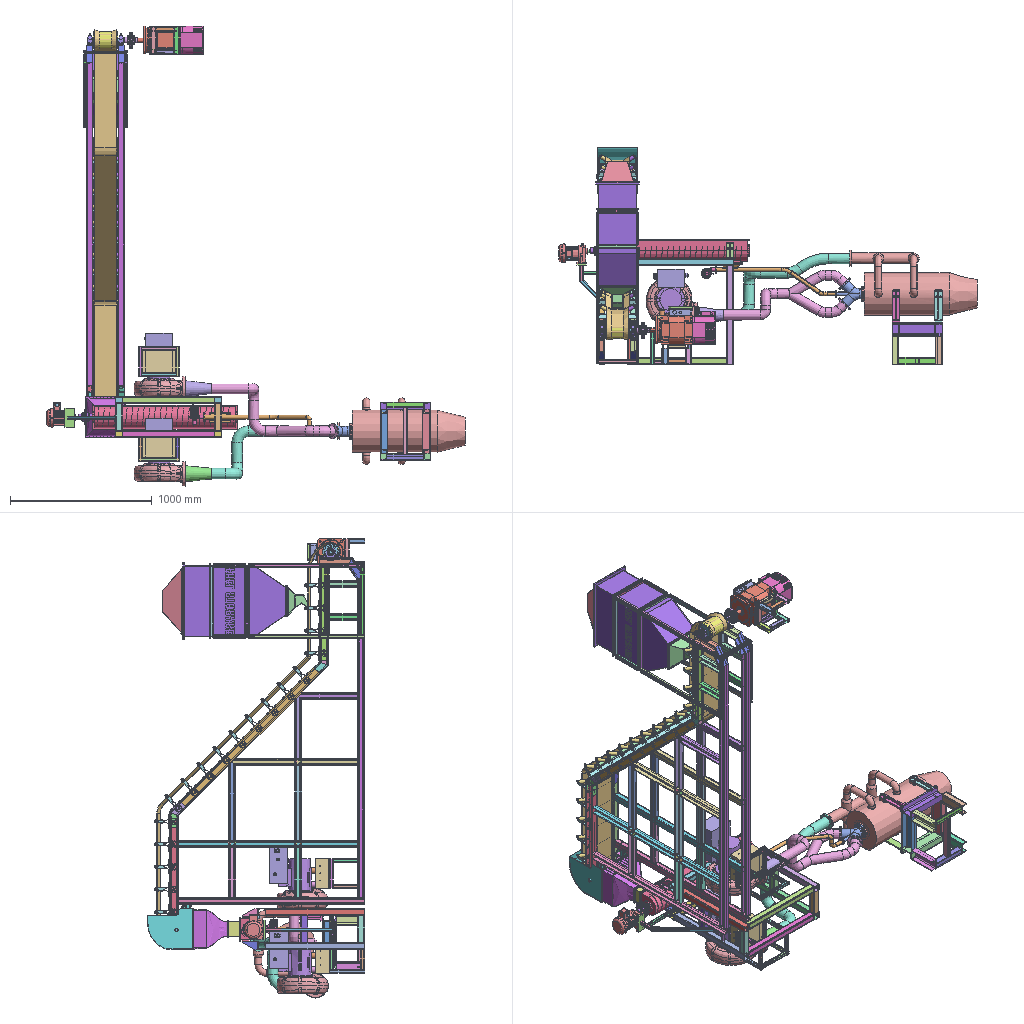Assembly | STEP file | 171 different items | 266 placed | box 2958 x 1534 x 3249 mm
Parts list (item | name | quantity | parent item | size | volume):
1 | 02288023_01 | x4 | in 02288023 | 52 x 34.1 x 52 mm | 26844 mm3
2 | 02288023_02 | x4 | in 02288023 | 140 x 38 x 80.599 mm | 93957 mm3
3 | Coal Storage | x1 | - | 1037 x 540 x 310 mm | 5068760 mm3
4 | Comveyor | x1 | - | - | -
5 | DIN 1026-1 U 30x15 1785506883170 | x1 | in Frame 1784900427749 | 15 x 30 x 530 mm | 112916 mm3
6 | DIN 1026-1 U 30x15 1785506933780 | x1 | in Frame 1784900427749 | 15 x 30 x 300 mm | 62027 mm3
7 | DIN 1026-1 U 30x15 1785506933862 | x1 | in Frame 1784900427749 | 15 x 30 x 530 mm | 112916 mm3
8 | DIN 1026-1 U 30x15 1785506933934 | x1 | in Frame 1784900427749 | 15 x 30 x 300 mm | 62027 mm3
9 | DIN 1026-1 U 30x15 1785506934014 | x1 | in Frame 1784900427749 | 15 x 30 x 530 mm | 112916 mm3
10 | DIN 1026-1 U 30x15 1785506934084 | x1 | in Frame 1784900427749 | 15 x 30 x 300 mm | 62027 mm3
11 | DIN 1026-1 U 30x15 1785506934163 | x1 | in Frame 1784900427749 | 15 x 30 x 530 mm | 112916 mm3
12 | DIN 1026-1 U 30x15 1785506934236 | x1 | in Frame 1784900427749 | 15 x 30 x 300 mm | 62027 mm3
13 | DIN 1026-1 U 30x15 1785507254409 | x1 | in Frame 1784900427749 | 15 x 30 x 815 mm | 180323 mm3
14 | DIN 1026-1 U 30x15 1785507254479 | x1 | in Frame 1784900427749 | 15 x 30 x 815 mm | 180323 mm3
15 | DIN 1026-1 U 30x15 1785507358854 | x1 | in Frame 1784900427749 | 15 x 30 x 815 mm | 180323 mm3
16 | DIN 1026-1 U 30x15 1785507358927 | x1 | in Frame 1784900427749 | 15 x 30 x 815 mm | 180323 mm3
17 | DIN 1026-1 U 30x15 1785507675323 | x1 | in Frame 1784900427749 | 15 x 30 x 470 mm | 103990 mm3
18 | DIN 1026-1 U 30x15 1785507675399 | x1 | in Frame 1784900427749 | 15 x 30 x 470 mm | 103990 mm3
19 | DIN 1026-1 U 30x15 1785507675476 | x1 | in Frame 1784900427749 | 15 x 30 x 270 mm | 59739 mm3
20 | DIN 1026-1 U 30x15 1785507904982 | x1 | in Frame 1784900427749 | 15 x 30 x 470 mm | 103990 mm3
21 | DIN 1026-1 U 30x15 1785507905050 | x1 | in Frame 1784900427749 | 15 x 30 x 470 mm | 103990 mm3
22 | DIN 1026-1 U 30x15 1785508252631 | x1 | in Frame 1784900427749 | 15 x 30 x 220 mm | 48676 mm3
23 | DIN 1026-1 U 30x15 1785508252702 | x1 | in Frame 1784900427749 | 15 x 30 x 220 mm | 48676 mm3
24 | DIN 1026-1 U 30x15 1785508276013 | x1 | in Frame 1784900427749 | 15 x 30 x 220 mm | 48676 mm3
25 | DIN 1026-1 U 30x15 1785508276077 | x1 | in Frame 1784900427749 | 15 x 30 x 220 mm | 48676 mm3
26 | DIN 1026-1 U 50 1785357045320 | x2 | in Frame 1784900427749, Frame 1784900427749_MIR1 | 38 x 50 x 1315 mm | 935965 mm3
27 | DIN 1026-1 U 50 1785357045389 | x2 | in Frame 1784900427749, Frame 1784900427749_MIR1 | 38 x 50 x 1265 mm | 900372 mm3
28 | DIN 1026-1 U 50 1785357045460 | x2 | in Frame 1784900427749, Frame 1784900427749_MIR1 | 38 x 50 x 885.962 mm | 617699 mm3
29 | DIN 1026-1 U 50 1785357045525 | x2 | in Frame 1784900427749, Frame 1784900427749_MIR1 | 38 x 50 x 417.981 mm | 284561 mm3
30 | DIN 1026-1 U 50 1785357045599 | x2 | in Frame 1784900427749, Frame 1784900427749_MIR1 | 38 x 50 x 204.153 mm | 145329 mm3
31 | DIN 1026-1 U 50 1785357074616 | x2 | in Frame 1784900427749, Frame 1784900427749_MIR1 | 38 x 50 x 953.851 mm | 646774 mm3
32 | DIN 1026-1 U 50 1785357074696 | x2 | in Frame 1784900427749, Frame 1784900427749_MIR1 | 38 x 50 x 1422 mm | 960658 mm3
33 | DIN 1026-1 U 50 1785357157092 | x2 | in Frame 1784900427749, Frame 1784900427749_MIR1 | 38 x 50 x 2278 mm | 1606422 mm3
34 | DIN 1026-1 U 50 1785357209510 | x2 | in Frame 1784900427749, Frame 1784900427749_MIR1 | 38 x 50 x 204.153 mm | 145329 mm3
35 | DIN 1026-1 U 65 1785352380286 | x1 | in Frame 1784900427749 | 42 x 65 x 667.157 mm | 598322 mm3
36 | DIN 1026-1 U 65 1785352380365 | x1 | in Frame 1784900427749 | 42 x 65 x 82.843 mm | 62132 mm3
37 | DIN 1026-1 U 65 1785352380440 | x1 | in Frame 1784900427749 | 42 x 65 x 82.843 mm | 62668 mm3
38 | DIN 1026-1 U 65 1785352380506 | x1 | in Frame 1784900427749 | 42 x 65 x 1334 mm | 1196644 mm3
39 | DIN 1026-1 U 65 1785352380582 | x1 | in Frame 1784900427749 | 42 x 65 x 109.767 mm | 85915 mm3
40 | DIN 1026-1 U 65 1785352380647 | x1 | in Frame 1784900427749 | 42 x 65 x 109.767 mm | 85915 mm3
41 | DIN 1026-1 U 65 1785352380714 | x1 | in Frame 1784900427749 | 42 x 65 x 707.157 mm | 633916 mm3
42 | DIN 1026-1 U 65 1785352674380 | x1 | in Frame 1784900427749 | 42 x 65 x 667.157 mm | 598322 mm3
43 | DIN 1026-1 U 65 1785352674453 | x1 | in Frame 1784900427749 | 42 x 65 x 82.843 mm | 62132 mm3
44 | DIN 1026-1 U 65 1785352674520 | x1 | in Frame 1784900427749 | 42 x 65 x 82.843 mm | 62668 mm3
45 | DIN 1026-1 U 65 1785352674597 | x1 | in Frame 1784900427749 | 42 x 65 x 1334 mm | 1196644 mm3
46 | DIN 1026-1 U 65 1785352674663 | x1 | in Frame 1784900427749 | 42 x 65 x 109.767 mm | 85915 mm3
47 | DIN 1026-1 U 65 1785352674731 | x1 | in Frame 1784900427749 | 42 x 65 x 109.767 mm | 85915 mm3
48 | DIN 1026-1 U 65 1785352674799 | x1 | in Frame 1784900427749 | 42 x 65 x 657.157 mm | 589289 mm3
49 | DIN 1026-1 U 65 1785415623013 | x1 | in Frame 1784900427749 | 42 x 65 x 234.079 mm | 194862 mm3
50 | DIN 1026-1 U 65 1785415623013_1 | x1 | in Frame 1784900427749_MIR1 | 42 x 65 x 234.079 mm | 194862 mm3
51 | DIN 1026-1 U 65 1785415623083 | x2 | in Frame 1784900427749, Frame 1784900427749_MIR1 | 42 x 65 x 155.66 mm | 122460 mm3
52 | DIN 1026-1 U 65 1785416005636 | x1 | in Frame 1784900427749_MIR1 | 42 x 65 x 120 mm | 74132 mm3
53 | DIN 1026-1 U 65 1785416005761 | x1 | in Frame 1784900427749_MIR1 | 42 x 65 x 150.668 mm | 136091 mm3
54 | DIN EN 10305-5 40 x 30 x 3 1785420022002 | x1 | in Frame 1784900427749 | 30 x 40 x 147.63 mm | 52459 mm3
55 | DIN EN 10305-5 40 x 30 x 3 1785420022002_1 | x1 | in Frame 1784900427749_MIR2 | 30 x 40 x 147.63 mm | 52459 mm3
56 | DIN EN 10305-5 40 x 30 x 3 1785420022083 | x1 | in Frame 1784900427749 | 30 x 40 x 19 mm | 6679 mm3
57 | DIN EN 10305-5 40 x 30 x 3 1785420022083_1 | x1 | in Frame 1784900427749_MIR2 | 30 x 40 x 19 mm | 6679 mm3
58 | DIN EN 10305-5 40 x 30 x 3 1785420075848 | x2 | in Frame 1784900427749, Frame 1784900427749_MIR2 | 30 x 40 x 115 mm | 41139 mm3
59 | DIN EN 10305-5 40 x 30 x 3 1785429634942 | x1 | in Frame 1784900427749 | 30 x 40 x 121.4 mm | 43429 mm3
60 | DIN EN 10305-5 40 x 30 x 3 1785429635057 | x1 | in Frame 1784900427749 | 30 x 40 x 121.4 mm | 43429 mm3
61 | DIN EN 10305-5 40 x 30 x 3 1785429668101 | x1 | in Frame 1784900427749 | 30 x 40 x 194.434 mm | 69555 mm3
62 | DIN EN 10305-5 40 x 30 x 3 1785429668188 | x1 | in Frame 1784900427749 | 30 x 40 x 194.434 mm | 69555 mm3
63 | DIN EN 10305-5 40 x 30 x 3 1785429742031 | x1 | in Frame 1784900427749 | 30 x 40 x 108 mm | 38635 mm3
64 | DIN EN 10305-5 40 x 30 x 3 1785429783133 | x1 | in Frame 1784900427749 | 30 x 40 x 108 mm | 38635 mm3
65 | DIN EN 10305-5 40 x 30 x 3 1785429807319 | x1 | in Frame 1784900427749 | 30 x 40 x 108 mm | 38635 mm3
66 | DIN EN 10305-5 40 x 30 x 3 1785429823978 | x1 | in Frame 1784900427749 | 30 x 40 x 108 mm | 38635 mm3
67 | DIN EN 10305-5 40 x 30 x 3 1785429986585 | x1 | in Frame 1784900427749 | 30 x 40 x 121.4 mm | 43429 mm3
68 | DIN EN 10305-5 40 x 30 x 3 1785429986663 | x1 | in Frame 1784900427749 | 30 x 40 x 122.222 mm | 43443 mm3
69 | FRAME BURNER | x1 | - | - | -
70 | Frame Combustor_1 | x1 | - | 350 x 230 x 412 mm | 696961 mm3
71 | Frame Idler_1 | x18 | in Frame Idler, 71 | 100 x 144.231 x 262 mm | 126128 mm3
72 | Frame Screw Feeder | x1 | - | 135 x 65 x 10 mm | 87750 mm3
73 | ISO 10799-2 25x25x3 1784905468546 | x1 | in Frame 1784900427749 | 25 x 25 x 236 mm | 56834 mm3
74 | ISO 10799-2 25x25x3 1784905468628 | x1 | in Frame 1784900427749 | 25 x 25 x 236 mm | 56834 mm3
75 | ISO 10799-2 25x25x3 1784905468712 | x1 | in Frame 1784900427749 | 25 x 25 x 208 mm | 50091 mm3
76 | ISO 10799-2 25x25x3 1784905468810 | x1 | in Frame 1784900427749 | 25 x 25 x 208 mm | 50091 mm3
77 | ISO 10799-2 25x25x3 1784905468899 | x1 | in Frame 1784900427749 | 25 x 25 x 222.2 mm | 53511 mm3
78 | ISO 10799-2 25x25x3 1784905468980 | x1 | in Frame 1784900427749 | 25 x 25 x 222.2 mm | 53511 mm3
79 | ISO 10799-2 25x25x3 1784905469066 | x1 | in Frame 1784900427749 | 25 x 25 x 222.2 mm | 53511 mm3
80 | ISO 10799-2 25x25x3 1784905469144 | x1 | in Frame 1784900427749 | 25 x 25 x 222.2 mm | 53511 mm3
81 | ISO 10799-2 25x25x3 1784905614519 | x1 | in Frame 1784900427749 | 25 x 25 x 236 mm | 56834 mm3
82 | ISO 10799-2 25x25x3 1784905614596 | x1 | in Frame 1784900427749 | 25 x 25 x 236 mm | 56834 mm3
83 | ISO 10799-2 25x25x3 1784906820603 | x1 | in Frame 1784900427749 | 25 x 25 x 236 mm | 56834 mm3
84 | ISO 10799-2 25x25x3 1784906820679 | x1 | in Frame 1784900427749 | 25 x 25 x 261 mm | 62855 mm3
85 | ISO 10799-2 25x25x3 1784906820767 | x1 | in Frame 1784900427749 | 25 x 25 x 158 mm | 38050 mm3
86 | ISO 10799-2 25x25x3 1784906820847 | x1 | in Frame 1784900427749 | 25 x 25 x 158 mm | 38050 mm3
87 | ISO 10799-2 25x25x3 1784906820939 | x1 | in Frame 1784900427749 | 25 x 25 x 245 mm | 59002 mm3
88 | ISO 10799-2 25x25x3 1784906821018 | x1 | in Frame 1784900427749 | 25 x 25 x 245 mm | 59002 mm3
89 | ISO 10799-2 25x25x3 1784906821110 | x1 | in Frame 1784900427749 | 25 x 25 x 195.176 mm | 47003 mm3
90 | ISO 10799-2 25x25x3 1784906821206 | x1 | in Frame 1784900427749 | 25 x 25 x 195.176 mm | 47003 mm3
91 | ISO 10799-2 25x25x3 1784906821283 | x1 | in Frame 1784900427749 | 25 x 25 x 141 mm | 33956 mm3
92 | ISO 10799-2 25x25x3 1784906821371 | x1 | in Frame 1784900427749 | 25 x 25 x 141 mm | 33956 mm3
93 | ISO 10799-2 25x25x3 1784906852780 | x1 | in Frame 1784900427749 | 25 x 25 x 236 mm | 56834 mm3
94 | ISO 10799-2 25x25x3 1784907954146 | x1 | in Frame 1784900427749 | 25 x 25 x 115.036 mm | 26491 mm3
95 | ISO 10799-2 25x25x3 1784907954226 | x1 | in Frame 1784900427749 | 25 x 25 x 504.794 mm | 118438 mm3
96 | ISO 10799-2 25x25x3 1784907954311 | x1 | in Frame 1784900427749 | 25 x 25 x 113.072 mm | 24220 mm3
97 | ISO 10799-2 25x25x3 1784907954397 | x1 | in Frame 1784900427749 | 25 x 25 x 101.928 mm | 21536 mm3
98 | ISO 10799-2 25x25x3 1784908143849 | x1 | in Frame 1784900427749 | 25 x 25 x 277.531 mm | 66836 mm3
99 | ISO 10799-2 25x25x3 1784908143949 | x1 | in Frame 1784900427749 | 25 x 72.5 x 72.5 mm | 22697 mm3
100 | ISO 10799-2 25x25x3 1784908144036 | x1 | in Frame 1784900427749 | 25 x 25 x 164.089 mm | 39516 mm3
101 | ISO 10799-2 50x30x3 1784900903573 | x1 | in Frame 1784900427749 | 30 x 50 x 332 mm | 139713 mm3
102 | ISO 657-2 50x 40x 5 1784900831893 | x1 | in Frame 1784900427749 | 40 x 50 x 260 mm | 110109 mm3
103 | ISO 657-2 50x 40x 5 1784900831971 | x1 | in Frame 1784900427749 | 40 x 50 x 260 mm | 110109 mm3
104 | ISO 657_11 CH 100 x 10 1784900428948 | x1 | in Frame 1784900427749 | 50 x 100 x 350 mm | 458586 mm3
105 | ISO 657_11 CH 100 x 10 1784900429010 | x1 | in Frame 1784900427749 | 50 x 100 x 350 mm | 458586 mm3
106 | ISO 657_11 CH 100 x 10 1784900456176 | x1 | in Frame 1784900427749 | 50 x 100 x 312 mm | 408796 mm3
107 | ISO 657_11 CH 100 x 10 1784900456235 | x1 | in Frame 1784900427749 | 50 x 100 x 312 mm | 408796 mm3
108 | ISO 657_11 CH 80 x 8 1784900614284 | x1 | in Frame 1784900427749 | 45 x 80 x 200 mm | 209713 mm3
109 | ISO 657_11 CH 80 x 8 1784900614355 | x1 | in Frame 1784900427749 | 45 x 80 x 200 mm | 209713 mm3
110 | ISO 657_11 CH 80 x 8 1784900725769 | x1 | in Frame 1784900427749 | 45 x 80 x 200 mm | 209713 mm3
111 | ISO 657_11 CH 80 x 8 1784900743666 | x1 | in Frame 1784900427749 | 45 x 80 x 200 mm | 209713 mm3
112 | Idler | x18 | in Frame Idler, 71 | 25 x 61.651 x 253.902 mm | 75095 mm3
113 | Idler 2 | x18 | in Frame Idler, 71 | 22 x 22 x 92.169 mm | 30779 mm3
114 | Idler 3 | x1 | in Frame Idler | 48.012 x 48.012 x 191.5 mm | 302346 mm3
115 | Idler 3_1 | x17 | in 71 | 48.012 x 48.012 x 194 mm | 302460 mm3
116 | JIS G 3466 50 x 50 x 3,2 1784903928658 | x1 | in Frame 1784900427749 | 50 x 50 x 750 mm | 429502 mm3
117 | JIS G 3466 50 x 50 x 3,2 1784903928729 | x1 | in Frame 1784900427749 | 50 x 50 x 750 mm | 429502 mm3
118 | JIS G 3466 50 x 50 x 3,2 1784904005805 | x1 | in Frame 1784900427749 | 50 x 50 x 698.813 mm | 400189 mm3
119 | JIS G 3466 50 x 50 x 3,2 1784904005875 | x1 | in Frame 1784900427749 | 50 x 50 x 698.813 mm | 400189 mm3
120 | JIS G 3466 50 x 50 x 3,2 1784904132541 | x1 | in Frame 1784900427749 | 50 x 50 x 698.813 mm | 400189 mm3
121 | JIS G 3466 50 x 50 x 3,2 1784904132614 | x1 | in Frame 1784900427749 | 50 x 50 x 698.813 mm | 400189 mm3
122 | JIS G 3466 50 x 50 x 3,2 1784904367085 | x1 | in Frame 1784900427749 | 50 x 50 x 650 mm | 372235 mm3
123 | JIS G 3466 50 x 50 x 3,2 1784904367151 | x1 | in Frame 1784900427749 | 50 x 50 x 650 mm | 372235 mm3
124 | JIS G 3466 50 x 50 x 3,2 1784904759157 | x1 | in Frame 1784900427749 | 50 x 50 x 190 mm | 108807 mm3
125 | JIS G 3466 50 x 50 x 3,2 1784904759236 | x1 | in Frame 1784900427749 | 50 x 50 x 190 mm | 108807 mm3
126 | JIS G 3466 50 x 50 x 3,2 1784905045251 | x1 | in Frame 1784900427749 | 50 x 50 x 190 mm | 108807 mm3
127 | JIS G 3466 50 x 50 x 3,2 1784905045315 | x1 | in Frame 1784900427749 | 50 x 50 x 190 mm | 108807 mm3
128 | Pipe Blower | x1 | - | 895.643 x 351.015 x 390.2 mm | 1112047 mm3
129 | Pipe Coal Feder | x1 | - | 850.746 x 236.073 x 160 mm | 290347 mm3
130 | Pipe Primary Air | x1 | - | 200 x 219.345 x 110.2 mm | 292078 mm3
131 | Pipe Secondary Air | x1 | - | 894.178 x 498.319 x 396.2 mm | 1004360 mm3
132 | Pulley | x2 | - | 124 x 124 x 280 mm | 525359 mm3
133 | Pulverized Coal Burner | x1 | - | 900 x 458.1 x 470 mm | 45029265 mm3
134 | Reducer Primary Air | x1 | - | 185 x 174 x 174 mm | 225205 mm3
135 | Reducer Secondary | x1 | - | 185 x 174 x 174 mm | 229980 mm3
136 | Rolling bearing 70000AC 71905 AC GB_T 292 | x1 | in Bearing1 | 9 x 42 x 42 mm | 5353 mm3
137 | Rolling bearing 70000C 7004 C GB_T 292 | x1 | in Bearing2 | 12 x 42 x 42 mm | 8552 mm3
138 | Rubber Conveyor | x1 | - | 1297 x 2817 x 170 mm | 2976993 mm3
139 | Screew Feeder | x1 | - | 290 x 822.474 x 1075 mm | 4769697 mm3
140 | Skeleton 1784900427750 | x1 | in Frame 1784900427749 | - | -
141 | Swirl | x1 | - | 24 x 70.2 x 70.2 mm | 25661 mm3
142 | a-hp_225_37-140_3_0_01 | x2 | in a-hp_225_37-140_3_0 | 213 x 100 x 286 mm | 4101760 mm3
143 | a-hp_225_37-140_3_0_02 | x2 | in a-hp_225_37-140_3_0 | 233 x 251 x 200 mm | 5912482 mm3
144 | a-hp_225_37-140_3_0_03 | x2 | in a-hp_225_37-140_3_0 | 0.1 x 25 x 40 mm | 85.323 mm3
145 | a-hp_225_37-140_3_0_04 | x2 | in a-hp_225_37-140_3_0 | 174 x 361.133 x 361.501 mm | 10635738 mm3
146 | a-hp_225_37-140_3_0_05 | x2 | in a-hp_225_37-140_3_0 | 1.5 x 180 x 180 mm | 24200 mm3
147 | a-hp_225_37-140_3_0_06 | x2 | in a-hp_225_37-140_3_0 | 40 x 30 x 40 mm | 37699 mm3
148 | a-hp_225_37-140_3_0_07 | x2 | in a-hp_225_37-140_3_0 | 40 x 30 x 40 mm | 37699 mm3
149 | a-hp_225_37-140_3_0_08 | x2 | in a-hp_225_37-140_3_0 | 40 x 30 x 40 mm | 37699 mm3
150 | a-hp_225_37-140_3_0_09 | x2 | in a-hp_225_37-140_3_0 | 40 x 30 x 40 mm | 37699 mm3
151 | a-hp_225_37-140_3_0_10 | x2 | in a-hp_225_37-140_3_0 | 283 x 133 x 242 mm | 6782742 mm3
152 | basic_gh_motor_gh1_01 | x1 | in basic_gh_motor_gh1 | 41.25 x 21.6 x 21.6 mm | 12015 mm3
153 | basic_gh_motor_gh1_02 | x1 | in basic_gh_motor_gh1 | 203.75 x 137 x 177.5 mm | 2157267 mm3
154 | basic_gh_motor_gh1_03 | x1 | in basic_gh_motor_gh1 | 5.16 x 5.16 x 62.27 mm | 1302 mm3
155 | basic_gh_motor_gh1_04 | x1 | in basic_gh_motor_gh1 | 5.16 x 5.16 x 62.27 mm | 1302 mm3
156 | basic_gh_motor_gh1_05 | x1 | in basic_gh_motor_gh1 | 5.16 x 5.16 x 62.27 mm | 1302 mm3
157 | basic_gh_motor_gh1_06 | x1 | in basic_gh_motor_gh1 | 5.16 x 5.16 x 62.27 mm | 1302 mm3
158 | basic_gh_motor_gh1_07 | x1 | in basic_gh_motor_gh1 | 6.2 x 15.48 x 6.2 mm | 467.352 mm3
159 | basic_gh_motor_gh1_08 | x1 | in basic_gh_motor_gh1 | 6.2 x 15.48 x 6.2 mm | 467.352 mm3
160 | basic_gh_motor_gh1_09 | x1 | in basic_gh_motor_gh1 | 6.2 x 6.2 x 15.48 mm | 467.352 mm3
161 | basic_gh_motor_gh1_10 | x1 | in basic_gh_motor_gh1 | 6.2 x 6.2 x 15.48 mm | 467.352 mm3
162 | basic_gh_motor_gh1_11 | x1 | in basic_gh_motor_gh1 | 20.64 x 25.8 x 20.64 mm | 7104 mm3
163 | basic_gh_motor_gh1_12 | x1 | in basic_gh_motor_gh1 | 18 x 10.969 x 18 mm | 2099 mm3
164 | basic_gh_motor_gh1_13 | x1 | in basic_gh_motor_gh1 | 15.57 x 3.3 x 15.57 mm | 160.112 mm3
165 | basic_gh_motor_gh1_14 | x1 | in basic_gh_motor_gh1 | 46.5 x 12.371 x 24.915 mm | 1397 mm3
166 | basic_gh_motor_gh1_15 | x1 | in basic_gh_motor_gh1 | 18.75 x 7.973 x 19.478 mm | 421.53 mm3
167 | basic_gh_motor_gh1_16 | x1 | in basic_gh_motor_gh1 | 31.17 x 0.11 x 25.975 mm | 53.443 mm3
168 | couplings_1020t20-13 | x1 | - | 99.2 x 112 x 112 mm | 175171 mm3
169 | couplings_22222 | x1 | - | 99.2 x 112 x 112 mm | 164503 mm3
170 | motor_qs-100s-6_2-2600-360-87-b35-a | x1 | - | 200 x 266.5 x 480 mm | 10312452 mm3
171 | u71hl-024km-41 | x1 | - | 93.697 x 150.3 x 101.919 mm | 187964 mm3